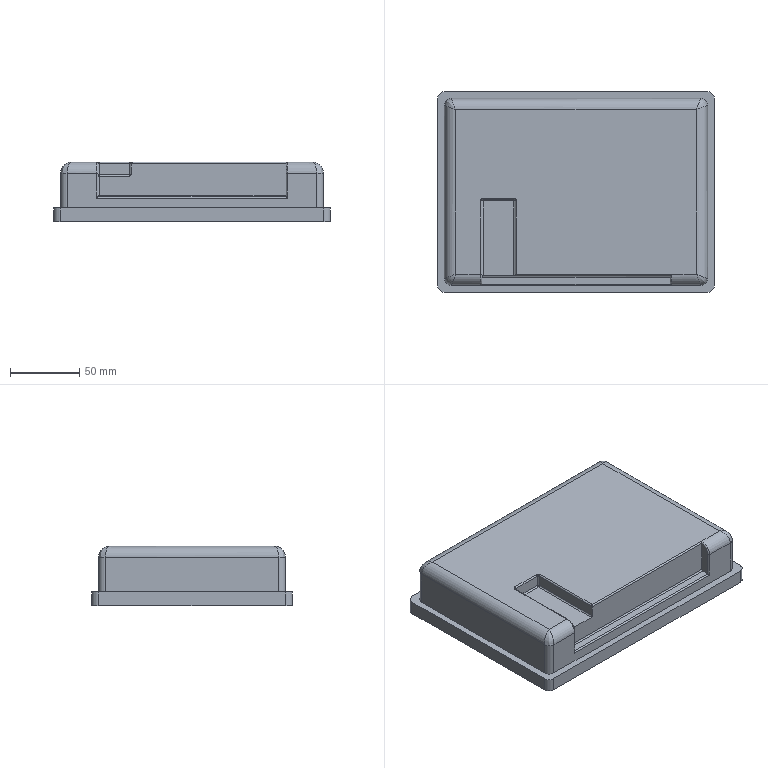Part | SolidWorks | features ICE 5, Fillet 3, Extrusion 1 | 1 solid | 70 faces | box 200 x 145 x 43 mm | volume 1064774 mm3 | cylinder 31 | plane 28 | torus 5 | spline 4 | sphere 2 | commonest cylinder face diameters 2 x14 10 x12 16 x5